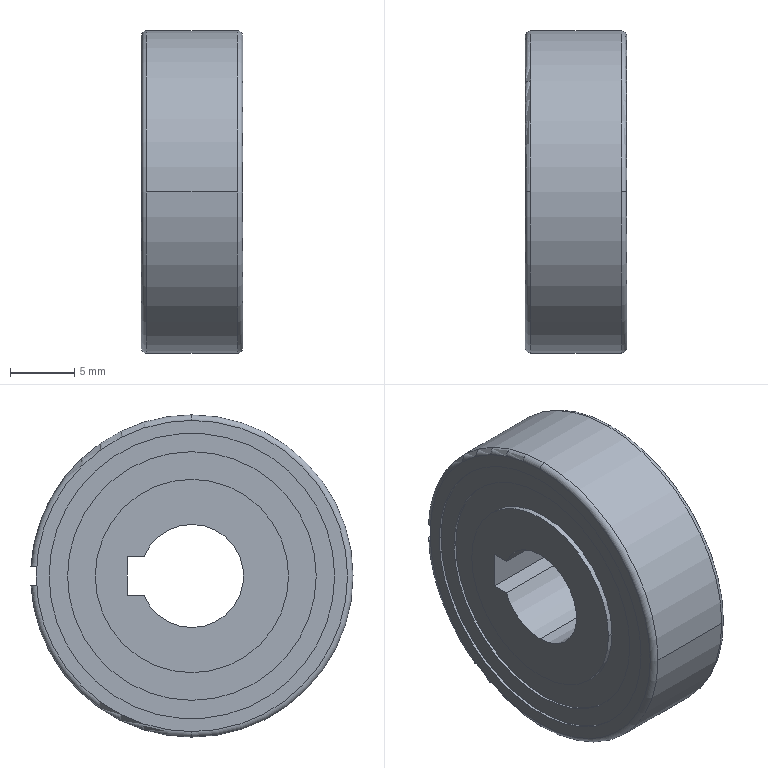Part | SolidWorks | features ICE 3, BaseBody 1, Scale 1 | 1 solid | 37 faces | box 7.854 x 24.97 x 24.99 mm | volume 3293 mm3 | cylinder 17 | plane 14 | torus 6 | commonest cylinder face diameters 14.994 x4 19.278 x4 22.134 x4 8 x3 24.99 x2
STEP:
#1=CARTESIAN_POINT('',(-3.927,-0.02811,4.));
#2=VERTEX_POINT('',#1);
#3=CARTESIAN_POINT('',(-3.927,-0.02811,-4.));
#4=VERTEX_POINT('',#3);
#5=CARTESIAN_POINT('',(-3.927,-0.02811,0.));
#6=DIRECTION('',(1.,0.,0.));
#7=DIRECTION('',(0.,0.,1.));
#8=AXIS2_PLACEMENT_3D('',#5,#6,#7);
#9=CIRCLE('',#8,4.);
#10=EDGE_CURVE('',#2,#4,#9,.T.);
#11=ORIENTED_EDGE('',*,*,#10,.F.);
#12=CARTESIAN_POINT('',(3.927,-0.02811,4.));
#13=VERTEX_POINT('',#12);
#14=CARTESIAN_POINT('',(-19.691,-0.02811,4.));
#15=DIRECTION('',(1.,0.,0.));
#16=VECTOR('',#15,1000.);
#17=LINE('',#14,#16);
#18=EDGE_CURVE('',#2,#13,#17,.T.);
#19=ORIENTED_EDGE('',*,*,#18,.T.);
#20=CARTESIAN_POINT('',(3.927,-0.02811,-4.));
#21=VERTEX_POINT('',#20);
#22=CARTESIAN_POINT('',(3.927,-0.02811,0.));
#23=DIRECTION('',(1.,0.,0.));
#24=DIRECTION('',(0.,0.,-1.));
#25=AXIS2_PLACEMENT_3D('',#22,#23,#24);
#26=CIRCLE('',#25,4.);
#27=EDGE_CURVE('',#13,#21,#26,.T.);
#28=ORIENTED_EDGE('',*,*,#27,.T.);
#29=CARTESIAN_POINT('',(-19.691,-0.02811,-4.));
#30=DIRECTION('',(1.,0.,0.));
#31=VECTOR('',#30,1000.);
#32=LINE('',#29,#31);
#33=EDGE_CURVE('',#4,#21,#32,.T.);
#34=ORIENTED_EDGE('',*,*,#33,.F.);
#35=EDGE_LOOP('',(#11,#19,#28,#34));
#36=FACE_OUTER_BOUND('',#35,.T.);
#37=CARTESIAN_POINT('',(-19.691,-0.02811,0.));
#38=DIRECTION('',(1.,0.,0.));
#39=DIRECTION('',(0.,0.,-1.));
#40=AXIS2_PLACEMENT_3D('',#37,#38,#39);
#41=CYLINDRICAL_SURFACE('',#40,4.);
#42=ADVANCED_FACE('',(#36),#41,.F.);
#43=CARTESIAN_POINT('',(-3.927,3.68,-1.5));
#44=VERTEX_POINT('',#43);
#45=CARTESIAN_POINT('',(-3.927,-0.02811,0.));
#46=DIRECTION('',(1.,0.,0.));
#47=DIRECTION('',(0.,0.,1.));
#48=AXIS2_PLACEMENT_3D('',#45,#46,#47);
#49=CIRCLE('',#48,4.);
#50=EDGE_CURVE('',#4,#44,#49,.T.);
#51=ORIENTED_EDGE('',*,*,#50,.F.);
#52=ORIENTED_EDGE('',*,*,#33,.T.);
#53=CARTESIAN_POINT('',(3.927,3.68,-1.5));
#54=VERTEX_POINT('',#53);
#55=CARTESIAN_POINT('',(3.927,-0.02811,0.));
#56=DIRECTION('',(1.,0.,0.));
#57=DIRECTION('',(0.,0.,-1.));
#58=AXIS2_PLACEMENT_3D('',#55,#56,#57);
#59=CIRCLE('',#58,4.);
#60=EDGE_CURVE('',#21,#54,#59,.T.);
#61=ORIENTED_EDGE('',*,*,#60,.T.);
#62=CARTESIAN_POINT('',(-19.691,3.68,-1.5));
#63=DIRECTION('',(-1.,0.,0.));
#64=VECTOR('',#63,1000.);
#65=LINE('',#62,#64);
#66=EDGE_CURVE('',#54,#44,#65,.T.);
#67=ORIENTED_EDGE('',*,*,#66,.T.);
#68=EDGE_LOOP('',(#51,#52,#61,#67));
#69=FACE_OUTER_BOUND('',#68,.T.);
#70=CARTESIAN_POINT('',(-19.691,-0.02811,0.));
#71=DIRECTION('',(1.,0.,0.));
#72=DIRECTION('',(0.,0.,-1.));
#73=AXIS2_PLACEMENT_3D('',#70,#71,#72);
#74=CYLINDRICAL_SURFACE('',#73,4.);
#75=ADVANCED_FACE('',(#69),#74,.F.);
#76=CARTESIAN_POINT('',(3.927,11.039,0.));
#77=VERTEX_POINT('',#76);
#78=CARTESIAN_POINT('',(3.927,-11.095,0.));
#79=VERTEX_POINT('',#78);
#80=CARTESIAN_POINT('',(3.927,-0.02811,0.));
#81=DIRECTION('',(-1.,0.,0.));
#82=DIRECTION('',(0.,1.,0.));
#83=AXIS2_PLACEMENT_3D('',#80,#81,#82);
#84=CIRCLE('',#83,11.067);
#85=EDGE_CURVE('',#77,#79,#84,.T.);
#86=ORIENTED_EDGE('',*,*,#85,.T.);
#87=CARTESIAN_POINT('',(3.927,-0.02811,0.));
#88=DIRECTION('',(-1.,0.,0.));
#89=DIRECTION('',(0.,1.,0.));
#90=AXIS2_PLACEMENT_3D('',#87,#88,#89);
#91=CIRCLE('',#90,11.067);
#92=EDGE_CURVE('',#79,#77,#91,.T.);
#93=ORIENTED_EDGE('',*,*,#92,.T.);
#94=EDGE_LOOP('',(#86,#93));
#95=FACE_BOUND('',#94,.T.);
#96=CARTESIAN_POINT('',(3.927,12.038,0.));
#97=VERTEX_POINT('',#96);
#98=CARTESIAN_POINT('',(3.927,-0.02811,-12.067));
#99=VERTEX_POINT('',#98);
#100=CARTESIAN_POINT('',(3.927,-0.02811,0.));
#101=DIRECTION('',(-1.,0.,0.));
#102=DIRECTION('',(0.,1.,0.));
#103=AXIS2_PLACEMENT_3D('',#100,#101,#102);
#104=CIRCLE('',#103,12.067);
#105=EDGE_CURVE('',#97,#99,#104,.T.);
#106=ORIENTED_EDGE('',*,*,#105,.F.);
#107=CARTESIAN_POINT('',(3.927,-0.02811,12.067));
#108=VERTEX_POINT('',#107);
#109=CARTESIAN_POINT('',(3.927,-0.02811,0.));
#110=DIRECTION('',(-1.,0.,0.));
#111=DIRECTION('',(0.,1.,0.));
#112=AXIS2_PLACEMENT_3D('',#109,#110,#111);
#113=CIRCLE('',#112,12.067);
#114=EDGE_CURVE('',#108,#97,#113,.T.);
#115=ORIENTED_EDGE('',*,*,#114,.F.);
#116=CARTESIAN_POINT('',(3.927,-0.02811,0.));
#117=DIRECTION('',(-1.,0.,0.));
#118=DIRECTION('',(0.,1.,0.));
#119=AXIS2_PLACEMENT_3D('',#116,#117,#118);
#120=CIRCLE('',#119,12.067);
#121=EDGE_CURVE('',#99,#108,#120,.T.);
#122=ORIENTED_EDGE('',*,*,#121,.F.);
#123=EDGE_LOOP('',(#106,#115,#122));
#124=FACE_OUTER_BOUND('',#123,.T.);
#125=CARTESIAN_POINT('',(3.927,11.539,0.));
#126=DIRECTION('',(1.,0.,0.));
#127=DIRECTION('',(0.,1.,0.));
#128=AXIS2_PLACEMENT_3D('',#125,#126,#127);
#129=PLANE('',#128);
#130=ADVANCED_FACE('',(#95,#124),#129,.T.);
#131=CARTESIAN_POINT('',(3.731,11.039,0.));
#132=VERTEX_POINT('',#131);
#133=CARTESIAN_POINT('',(3.829,11.039,0.));
#134=DIRECTION('',(-1.,0.,0.));
#135=VECTOR('',#134,1000.);
#136=LINE('',#133,#135);
#137=EDGE_CURVE('',#77,#132,#136,.T.);
#138=ORIENTED_EDGE('',*,*,#137,.T.);
#139=CARTESIAN_POINT('',(3.731,-11.095,0.));
#140=VERTEX_POINT('',#139);
#141=CARTESIAN_POINT('',(3.731,-0.02811,0.));
#142=DIRECTION('',(-1.,0.,0.));
#143=DIRECTION('',(0.,1.,0.));
#144=AXIS2_PLACEMENT_3D('',#141,#142,#143);
#145=CIRCLE('',#144,11.067);
#146=EDGE_CURVE('',#132,#140,#145,.T.);
#147=ORIENTED_EDGE('',*,*,#146,.T.);
#148=CARTESIAN_POINT('',(3.829,-11.095,0.));
#149=DIRECTION('',(1.,0.,0.));
#150=VECTOR('',#149,1000.);
#151=LINE('',#148,#150);
#152=EDGE_CURVE('',#140,#79,#151,.T.);
#153=ORIENTED_EDGE('',*,*,#152,.T.);
#154=ORIENTED_EDGE('',*,*,#85,.F.);
#155=EDGE_LOOP('',(#138,#147,#153,#154));
#156=FACE_OUTER_BOUND('',#155,.T.);
#157=CARTESIAN_POINT('',(3.829,-0.02811,0.));
#158=DIRECTION('',(-1.,0.,0.));
#159=DIRECTION('',(0.,1.,0.));
#160=AXIS2_PLACEMENT_3D('',#157,#158,#159);
#161=CYLINDRICAL_SURFACE('',#160,11.067);
#162=ADVANCED_FACE('',(#156),#161,.F.);
#163=CARTESIAN_POINT('',(3.731,9.611,0.));
#164=VERTEX_POINT('',#163);
#165=CARTESIAN_POINT('',(3.731,-9.667,0.));
#166=VERTEX_POINT('',#165);
#167=CARTESIAN_POINT('',(3.731,-0.02811,0.));
#168=DIRECTION('',(-1.,0.,0.));
#169=DIRECTION('',(0.,1.,0.));
#170=AXIS2_PLACEMENT_3D('',#167,#168,#169);
#171=CIRCLE('',#170,9.639);
#172=EDGE_CURVE('',#164,#166,#171,.T.);
#173=ORIENTED_EDGE('',*,*,#172,.T.);
#174=CARTESIAN_POINT('',(3.731,-0.02811,0.));
#175=DIRECTION('',(-1.,0.,0.));
#176=DIRECTION('',(0.,1.,0.));
#177=AXIS2_PLACEMENT_3D('',#174,#175,#176);
#178=CIRCLE('',#177,9.639);
#179=EDGE_CURVE('',#166,#164,#178,.T.);
#180=ORIENTED_EDGE('',*,*,#179,.T.);
#181=EDGE_LOOP('',(#173,#180));
#182=FACE_BOUND('',#181,.T.);
#183=ORIENTED_EDGE('',*,*,#146,.F.);
#184=CARTESIAN_POINT('',(3.731,-0.02811,0.));
#185=DIRECTION('',(-1.,0.,0.));
#186=DIRECTION('',(0.,1.,0.));
#187=AXIS2_PLACEMENT_3D('',#184,#185,#186);
#188=CIRCLE('',#187,11.067);
#189=EDGE_CURVE('',#140,#132,#188,.T.);
#190=ORIENTED_EDGE('',*,*,#189,.F.);
#191=EDGE_LOOP('',(#183,#190));
#192=FACE_OUTER_BOUND('',#191,.T.);
#193=CARTESIAN_POINT('',(3.731,10.325,0.));
#194=DIRECTION('',(1.,0.,0.));
#195=DIRECTION('',(0.,1.,0.));
#196=AXIS2_PLACEMENT_3D('',#193,#194,#195);
#197=PLANE('',#196);
#198=ADVANCED_FACE('',(#182,#192),#197,.T.);
#199=CARTESIAN_POINT('',(3.534,9.611,0.));
#200=VERTEX_POINT('',#199);
#201=CARTESIAN_POINT('',(3.632,9.611,0.));
#202=DIRECTION('',(-1.,0.,0.));
#203=VECTOR('',#202,1000.);
#204=LINE('',#201,#203);
#205=EDGE_CURVE('',#164,#200,#204,.T.);
#206=ORIENTED_EDGE('',*,*,#205,.T.);
#207=CARTESIAN_POINT('',(3.534,-9.667,0.));
#208=VERTEX_POINT('',#207);
#209=CARTESIAN_POINT('',(3.534,-0.02811,0.));
#210=DIRECTION('',(-1.,0.,0.));
#211=DIRECTION('',(0.,1.,0.));
#212=AXIS2_PLACEMENT_3D('',#209,#210,#211);
#213=CIRCLE('',#212,9.639);
#214=EDGE_CURVE('',#200,#208,#213,.T.);
#215=ORIENTED_EDGE('',*,*,#214,.T.);
#216=CARTESIAN_POINT('',(3.632,-9.667,0.));
#217=DIRECTION('',(1.,0.,0.));
#218=VECTOR('',#217,1000.);
#219=LINE('',#216,#218);
#220=EDGE_CURVE('',#208,#166,#219,.T.);
#221=ORIENTED_EDGE('',*,*,#220,.T.);
#222=ORIENTED_EDGE('',*,*,#172,.F.);
#223=EDGE_LOOP('',(#206,#215,#221,#222));
#224=FACE_OUTER_BOUND('',#223,.T.);
#225=CARTESIAN_POINT('',(3.632,-0.02811,0.));
#226=DIRECTION('',(-1.,0.,0.));
#227=DIRECTION('',(0.,1.,0.));
#228=AXIS2_PLACEMENT_3D('',#225,#226,#227);
#229=CYLINDRICAL_SURFACE('',#228,9.639);
#230=ADVANCED_FACE('',(#224),#229,.F.);
#231=CARTESIAN_POINT('',(3.534,7.469,0.));
#232=VERTEX_POINT('',#231);
#233=CARTESIAN_POINT('',(3.534,-7.525,0.));
#234=VERTEX_POINT('',#233);
#235=CARTESIAN_POINT('',(3.534,-0.02811,0.));
#236=DIRECTION('',(-1.,0.,0.));
#237=DIRECTION('',(0.,1.,0.));
#238=AXIS2_PLACEMENT_3D('',#235,#236,#237);
#239=CIRCLE('',#238,7.497);
#240=EDGE_CURVE('',#232,#234,#239,.T.);
#241=ORIENTED_EDGE('',*,*,#240,.T.);
#242=CARTESIAN_POINT('',(3.534,-0.02811,0.));
#243=DIRECTION('',(-1.,0.,0.));
#244=DIRECTION('',(0.,1.,0.));
#245=AXIS2_PLACEMENT_3D('',#242,#243,#244);
#246=CIRCLE('',#245,7.497);
#247=EDGE_CURVE('',#234,#232,#246,.T.);
#248=ORIENTED_EDGE('',*,*,#247,.T.);
#249=EDGE_LOOP('',(#241,#248));
#250=FACE_BOUND('',#249,.T.);
#251=ORIENTED_EDGE('',*,*,#214,.F.);
#252=CARTESIAN_POINT('',(3.534,-0.02811,0.));
#253=DIRECTION('',(-1.,0.,0.));
#254=DIRECTION('',(0.,1.,0.));
#255=AXIS2_PLACEMENT_3D('',#252,#253,#254);
#256=CIRCLE('',#255,9.639);
#257=EDGE_CURVE('',#208,#200,#256,.T.);
#258=ORIENTED_EDGE('',*,*,#257,.F.);
#259=EDGE_LOOP('',(#251,#258));
#260=FACE_OUTER_BOUND('',#259,.T.);
#261=CARTESIAN_POINT('',(3.534,8.54,0.));
#262=DIRECTION('',(1.,0.,0.));
#263=DIRECTION('',(0.,1.,0.));
#264=AXIS2_PLACEMENT_3D('',#261,#262,#263);
#265=PLANE('',#264);
#266=ADVANCED_FACE('',(#250,#260),#265,.T.);
#267=CARTESIAN_POINT('',(3.927,7.469,0.));
#268=VERTEX_POINT('',#267);
#269=CARTESIAN_POINT('',(3.731,7.469,0.));
#270=DIRECTION('',(-1.,0.,0.));
#271=VECTOR('',#270,1000.);
#272=LINE('',#269,#271);
#273=EDGE_CURVE('',#268,#232,#272,.T.);
#274=ORIENTED_EDGE('',*,*,#273,.T.);
#275=ORIENTED_EDGE('',*,*,#247,.F.);
#276=CARTESIAN_POINT('',(3.927,-7.525,0.));
#277=VERTEX_POINT('',#276);
#278=CARTESIAN_POINT('',(3.731,-7.525,0.));
#279=DIRECTION('',(1.,0.,0.));
#280=VECTOR('',#279,1000.);
#281=LINE('',#278,#280);
#282=EDGE_CURVE('',#234,#277,#281,.T.);
#283=ORIENTED_EDGE('',*,*,#282,.T.);
#284=CARTESIAN_POINT('',(3.927,-0.02811,0.));
#285=DIRECTION('',(-1.,0.,0.));
#286=DIRECTION('',(0.,1.,0.));
#287=AXIS2_PLACEMENT_3D('',#284,#285,#286);
#288=CIRCLE('',#287,7.497);
#289=EDGE_CURVE('',#277,#268,#288,.T.);
#290=ORIENTED_EDGE('',*,*,#289,.T.);
#291=EDGE_LOOP('',(#274,#275,#283,#290));
#292=FACE_OUTER_BOUND('',#291,.T.);
#293=CARTESIAN_POINT('',(3.731,-0.02811,0.));
#294=DIRECTION('',(-1.,0.,0.));
#295=DIRECTION('',(0.,1.,0.));
#296=AXIS2_PLACEMENT_3D('',#293,#294,#295);
#297=CYLINDRICAL_SURFACE('',#296,7.497);
#298=ADVANCED_FACE('',(#292),#297,.T.);
#299=CARTESIAN_POINT('',(3.927,5.,-1.5));
#300=VERTEX_POINT('',#299);
#301=CARTESIAN_POINT('',(3.927,5.,-1.5));
#302=DIRECTION('',(0.,1.,0.));
#303=VECTOR('',#302,1000.);
#304=LINE('',#301,#303);
#305=EDGE_CURVE('',#54,#300,#304,.T.);
#306=ORIENTED_EDGE('',*,*,#305,.F.);
#307=ORIENTED_EDGE('',*,*,#60,.F.);
#308=ORIENTED_EDGE('',*,*,#27,.F.);
#309=CARTESIAN_POINT('',(3.927,3.68,1.5));
#310=VERTEX_POINT('',#309);
#311=CARTESIAN_POINT('',(3.927,-0.02811,0.));
#312=DIRECTION('',(1.,0.,0.));
#313=DIRECTION('',(0.,0.,-1.));
#314=AXIS2_PLACEMENT_3D('',#311,#312,#313);
#315=CIRCLE('',#314,4.);
#316=EDGE_CURVE('',#310,#13,#315,.T.);
#317=ORIENTED_EDGE('',*,*,#316,.F.);
#318=CARTESIAN_POINT('',(3.927,5.,1.5));
#319=VERTEX_POINT('',#318);
#320=CARTESIAN_POINT('',(3.927,5.,1.5));
#321=DIRECTION('',(0.,-1.,0.));
#322=VECTOR('',#321,1000.);
#323=LINE('',#320,#322);
#324=EDGE_CURVE('',#319,#310,#323,.T.);
#325=ORIENTED_EDGE('',*,*,#324,.F.);
#326=CARTESIAN_POINT('',(3.927,5.,1.5));
#327=DIRECTION('',(0.,0.,1.));
#328=VECTOR('',#327,1000.);
#329=LINE('',#326,#328);
#330=EDGE_CURVE('',#300,#319,#329,.T.);
#331=ORIENTED_EDGE('',*,*,#330,.F.);
#332=EDGE_LOOP('',(#306,#307,#308,#317,#325,#331));
#333=FACE_BOUND('',#332,.T.);
#334=CARTESIAN_POINT('',(3.927,-0.02811,0.));
#335=DIRECTION('',(-1.,0.,0.));
#336=DIRECTION('',(0.,1.,0.));
#337=AXIS2_PLACEMENT_3D('',#334,#335,#336);
#338=CIRCLE('',#337,7.497);
#339=EDGE_CURVE('',#268,#277,#338,.T.);
#340=ORIENTED_EDGE('',*,*,#339,.F.);
#341=ORIENTED_EDGE('',*,*,#289,.F.);
#342=EDGE_LOOP('',(#340,#341));
#343=FACE_OUTER_BOUND('',#342,.T.);
#344=CARTESIAN_POINT('',(3.927,6.612,0.));
#345=DIRECTION('',(1.,0.,0.));
#346=DIRECTION('',(0.,1.,0.));
#347=AXIS2_PLACEMENT_3D('',#344,#345,#346);
#348=PLANE('',#347);
#349=ADVANCED_FACE('',(#333,#343),#348,.T.);
#350=CARTESIAN_POINT('',(-3.534,7.469,0.));
#351=VERTEX_POINT('',#350);
#352=CARTESIAN_POINT('',(-3.927,7.469,0.));
#353=VERTEX_POINT('',#352);
#354=CARTESIAN_POINT('',(-3.731,7.469,0.));
#355=DIRECTION('',(-1.,0.,0.));
#356=VECTOR('',#355,1000.);
#357=LINE('',#354,#356);
#358=EDGE_CURVE('',#351,#353,#357,.T.);
#359=ORIENTED_EDGE('',*,*,#358,.T.);
#360=CARTESIAN_POINT('',(-3.927,-7.525,0.));
#361=VERTEX_POINT('',#360);
#362=CARTESIAN_POINT('',(-3.927,-0.02811,0.));
#363=DIRECTION('',(-1.,0.,0.));
#364=DIRECTION('',(0.,1.,0.));
#365=AXIS2_PLACEMENT_3D('',#362,#363,#364);
#366=CIRCLE('',#365,7.497);
#367=EDGE_CURVE('',#361,#353,#366,.T.);
#368=ORIENTED_EDGE('',*,*,#367,.F.);
#369=CARTESIAN_POINT('',(-3.534,-7.525,0.));
#370=VERTEX_POINT('',#369);
#371=CARTESIAN_POINT('',(-3.731,-7.525,0.));
#372=DIRECTION('',(1.,0.,0.));
#373=VECTOR('',#372,1000.);
#374=LINE('',#371,#373);
#375=EDGE_CURVE('',#361,#370,#374,.T.);
#376=ORIENTED_EDGE('',*,*,#375,.T.);
#377=CARTESIAN_POINT('',(-3.534,-0.02811,0.));
#378=DIRECTION('',(-1.,0.,0.));
#379=DIRECTION('',(0.,1.,0.));
#380=AXIS2_PLACEMENT_3D('',#377,#378,#379);
#381=CIRCLE('',#380,7.497);
#382=EDGE_CURVE('',#370,#351,#381,.T.);
#383=ORIENTED_EDGE('',*,*,#382,.T.);
#384=EDGE_LOOP('',(#359,#368,#376,#383));
#385=FACE_OUTER_BOUND('',#384,.T.);
#386=CARTESIAN_POINT('',(-3.731,-0.02811,0.));
#387=DIRECTION('',(-1.,0.,0.));
#388=DIRECTION('',(0.,1.,0.));
#389=AXIS2_PLACEMENT_3D('',#386,#387,#388);
#390=CYLINDRICAL_SURFACE('',#389,7.497);
#391=ADVANCED_FACE('',(#385),#390,.T.);
#392=CARTESIAN_POINT('',(-3.534,-0.02811,0.));
#393=DIRECTION('',(-1.,0.,0.));
#394=DIRECTION('',(0.,1.,0.));
#395=AXIS2_PLACEMENT_3D('',#392,#393,#394);
#396=CIRCLE('',#395,7.497);
#397=EDGE_CURVE('',#351,#370,#396,.T.);
#398=ORIENTED_EDGE('',*,*,#397,.F.);
#399=ORIENTED_EDGE('',*,*,#382,.F.);
#400=EDGE_LOOP('',(#398,#399));
#401=FACE_BOUND('',#400,.T.);
#402=CARTESIAN_POINT('',(-3.534,9.611,0.));
#403=VERTEX_POINT('',#402);
#404=CARTESIAN_POINT('',(-3.534,-9.667,0.));
#405=VERTEX_POINT('',#404);
#406=CARTESIAN_POINT('',(-3.534,-0.02811,0.));
#407=DIRECTION('',(-1.,0.,0.));
#408=DIRECTION('',(0.,1.,0.));
#409=AXIS2_PLACEMENT_3D('',#406,#407,#408);
#410=CIRCLE('',#409,9.639);
#411=EDGE_CURVE('',#403,#405,#410,.T.);
#412=ORIENTED_EDGE('',*,*,#411,.T.);
#413=CARTESIAN_POINT('',(-3.534,-0.02811,0.));
#414=DIRECTION('',(-1.,0.,0.));
#415=DIRECTION('',(0.,1.,0.));
#416=AXIS2_PLACEMENT_3D('',#413,#414,#415);
#417=CIRCLE('',#416,9.639);
#418=EDGE_CURVE('',#405,#403,#417,.T.);
#419=ORIENTED_EDGE('',*,*,#418,.T.);
#420=EDGE_LOOP('',(#412,#419));
#421=FACE_OUTER_BOUND('',#420,.T.);
#422=CARTESIAN_POINT('',(-3.534,8.54,0.));
#423=DIRECTION('',(-1.,0.,0.));
#424=DIRECTION('',(0.,0.,1.));
#425=AXIS2_PLACEMENT_3D('',#422,#423,#424);
#426=PLANE('',#425);
#427=ADVANCED_FACE('',(#401,#421),#426,.T.);
#428=CARTESIAN_POINT('',(-3.731,9.611,0.));
#429=VERTEX_POINT('',#428);
#430=CARTESIAN_POINT('',(-3.632,9.611,0.));
#431=DIRECTION('',(-1.,0.,0.));
#432=VECTOR('',#431,1000.);
#433=LINE('',#430,#432);
#434=EDGE_CURVE('',#403,#429,#433,.T.);
#435=ORIENTED_EDGE('',*,*,#434,.T.);
#436=CARTESIAN_POINT('',(-3.731,-9.667,0.));
#437=VERTEX_POINT('',#436);
#438=CARTESIAN_POINT('',(-3.731,-0.02811,0.));
#439=DIRECTION('',(-1.,0.,0.));
#440=DIRECTION('',(0.,1.,0.));
#441=AXIS2_PLACEMENT_3D('',#438,#439,#440);
#442=CIRCLE('',#441,9.639);
#443=EDGE_CURVE('',#429,#437,#442,.T.);
#444=ORIENTED_EDGE('',*,*,#443,.T.);
#445=CARTESIAN_POINT('',(-3.632,-9.667,0.));
#446=DIRECTION('',(1.,0.,0.));
#447=VECTOR('',#446,1000.);
#448=LINE('',#445,#447);
#449=EDGE_CURVE('',#437,#405,#448,.T.);
#450=ORIENTED_EDGE('',*,*,#449,.T.);
#451=ORIENTED_EDGE('',*,*,#411,.F.);
#452=EDGE_LOOP('',(#435,#444,#450,#451));
#453=FACE_OUTER_BOUND('',#452,.T.);
#454=CARTESIAN_POINT('',(-3.632,-0.02811,0.));
#455=DIRECTION('',(-1.,0.,0.));
#456=DIRECTION('',(0.,1.,0.));
#457=AXIS2_PLACEMENT_3D('',#454,#455,#456);
#458=CYLINDRICAL_SURFACE('',#457,9.639);
#459=ADVANCED_FACE('',(#453),#458,.F.);
#460=ORIENTED_EDGE('',*,*,#443,.F.);
#461=CARTESIAN_POINT('',(-3.731,-0.02811,0.));
#462=DIRECTION('',(-1.,0.,0.));
#463=DIRECTION('',(0.,1.,0.));
#464=AXIS2_PLACEMENT_3D('',#461,#462,#463);
#465=CIRCLE('',#464,9.639);
#466=EDGE_CURVE('',#437,#429,#465,.T.);
#467=ORIENTED_EDGE('',*,*,#466,.F.);
#468=EDGE_LOOP('',(#460,#467));
#469=FACE_BOUND('',#468,.T.);
#470=CARTESIAN_POINT('',(-3.731,11.039,0.));
#471=VERTEX_POINT('',#470);
#472=CARTESIAN_POINT('',(-3.731,-11.095,0.));
#473=VERTEX_POINT('',#472);
#474=CARTESIAN_POINT('',(-3.731,-0.02811,0.));
#475=DIRECTION('',(-1.,0.,0.));
#476=DIRECTION('',(0.,1.,0.));
#477=AXIS2_PLACEMENT_3D('',#474,#475,#476);
#478=CIRCLE('',#477,11.067);
#479=EDGE_CURVE('',#471,#473,#478,.T.);
#480=ORIENTED_EDGE('',*,*,#479,.T.);
#481=CARTESIAN_POINT('',(-3.731,-0.02811,0.));
#482=DIRECTION('',(-1.,0.,0.));
#483=DIRECTION('',(0.,1.,0.));
#484=AXIS2_PLACEMENT_3D('',#481,#482,#483);
#485=CIRCLE('',#484,11.067);
#486=EDGE_CURVE('',#473,#471,#485,.T.);
#487=ORIENTED_EDGE('',*,*,#486,.T.);
#488=EDGE_LOOP('',(#480,#487));
#489=FACE_OUTER_BOUND('',#488,.T.);
#490=CARTESIAN_POINT('',(-3.731,10.325,0.));
#491=DIRECTION('',(-1.,0.,0.));
#492=DIRECTION('',(0.,0.,1.));
#493=AXIS2_PLACEMENT_3D('',#490,#491,#492);
#494=PLANE('',#493);
#495=ADVANCED_FACE('',(#469,#489),#494,.T.);
#496=CARTESIAN_POINT('',(-3.927,11.039,0.));
#497=VERTEX_POINT('',#496);
#498=CARTESIAN_POINT('',(-3.829,11.039,0.));
#499=DIRECTION('',(-1.,0.,0.));
#500=VECTOR('',#499,1000.);
#501=LINE('',#498,#500);
#502=EDGE_CURVE('',#471,#497,#501,.T.);
#503=ORIENTED_EDGE('',*,*,#502,.T.);
#504=CARTESIAN_POINT('',(-3.927,-11.095,0.));
#505=VERTEX_POINT('',#504);
#506=CARTESIAN_POINT('',(-3.927,-0.02811,0.));
#507=DIRECTION('',(-1.,0.,0.));
#508=DIRECTION('',(0.,1.,0.));
#509=AXIS2_PLACEMENT_3D('',#506,#507,#508);
#510=CIRCLE('',#509,11.067);
#511=EDGE_CURVE('',#497,#505,#510,.T.);
#512=ORIENTED_EDGE('',*,*,#511,.T.);
#513=CARTESIAN_POINT('',(-3.829,-11.095,0.));
#514=DIRECTION('',(1.,0.,0.));
#515=VECTOR('',#514,1000.);
#516=LINE('',#513,#515);
#517=EDGE_CURVE('',#505,#473,#516,.T.);
#518=ORIENTED_EDGE('',*,*,#517,.T.);
#519=ORIENTED_EDGE('',*,*,#479,.F.);
#520=EDGE_LOOP('',(#503,#512,#518,#519));
#521=FACE_OUTER_BOUND('',#520,.T.);
#522=CARTESIAN_POINT('',(-3.829,-0.02811,0.));
#523=DIRECTION('',(-1.,0.,0.));
#524=DIRECTION('',(0.,1.,0.));
#525=AXIS2_PLACEMENT_3D('',#522,#523,#524);
#526=CYLINDRICAL_SURFACE('',#525,11.067);
#527=ADVANCED_FACE('',(#521),#526,.F.);
#528=ORIENTED_EDGE('',*,*,#511,.F.);
#529=CARTESIAN_POINT('',(-3.927,-0.02811,0.));
#530=DIRECTION('',(-1.,0.,0.));
#531=DIRECTION('',(0.,1.,0.));
#532=AXIS2_PLACEMENT_3D('',#529,#530,#531);
#533=CIRCLE('',#532,11.067);
#534=EDGE_CURVE('',#505,#497,#533,.T.);
#535=ORIENTED_EDGE('',*,*,#534,.F.);
#536=EDGE_LOOP('',(#528,#535));
#537=FACE_BOUND('',#536,.T.);
#538=CARTESIAN_POINT('',(-3.927,12.038,0.));
#539=VERTEX_POINT('',#538);
#540=CARTESIAN_POINT('',(-3.927,-0.02811,-12.067));
#541=VERTEX_POINT('',#540);
#542=CARTESIAN_POINT('',(-3.927,-0.02811,0.));
#543=DIRECTION('',(-1.,0.,0.));
#544=DIRECTION('',(0.,1.,0.));
#545=AXIS2_PLACEMENT_3D('',#542,#543,#544);
#546=CIRCLE('',#545,12.067);
#547=EDGE_CURVE('',#539,#541,#546,.T.);
#548=ORIENTED_EDGE('',*,*,#547,.T.);
#549=CARTESIAN_POINT('',(-3.927,-0.02811,12.067));
#550=VERTEX_POINT('',#549);
#551=CARTESIAN_POINT('',(-3.927,-0.02811,0.));
#552=DIRECTION('',(-1.,0.,0.));
#553=DIRECTION('',(0.,1.,0.));
#554=AXIS2_PLACEMENT_3D('',#551,#552,#553);
#555=CIRCLE('',#554,12.067);
#556=EDGE_CURVE('',#541,#550,#555,.T.);
#557=ORIENTED_EDGE('',*,*,#556,.T.);
#558=CARTESIAN_POINT('',(-3.927,-0.02811,0.));
#559=DIRECTION('',(-1.,0.,0.));
#560=DIRECTION('',(0.,1.,0.));
#561=AXIS2_PLACEMENT_3D('',#558,#559,#560);
#562=CIRCLE('',#561,12.067);
#563=EDGE_CURVE('',#550,#539,#562,.T.);
#564=ORIENTED_EDGE('',*,*,#563,.T.);
#565=EDGE_LOOP('',(#548,#557,#564));
#566=FACE_OUTER_BOUND('',#565,.T.);
#567=CARTESIAN_POINT('',(-3.927,11.539,0.));
#568=DIRECTION('',(-1.,0.,0.));
#569=DIRECTION('',(0.,0.,1.));
#570=AXIS2_PLACEMENT_3D('',#567,#568,#569);
#571=PLANE('',#570);
#572=ADVANCED_FACE('',(#537,#566),#571,.T.);
#573=CARTESIAN_POINT('',(-3.499,-0.02811,12.495));
#574=VERTEX_POINT('',#573);
#575=CARTESIAN_POINT('',(-3.499,-0.02811,12.067));
#576=DIRECTION('',(0.,-1.,0.));
#577=DIRECTION('',(0.,0.,1.));
#578=AXIS2_PLACEMENT_3D('',#575,#576,#577);
#579=CIRCLE('',#578,0.4284);
#580=EDGE_CURVE('',#574,#550,#579,.T.);
#581=ORIENTED_EDGE('',*,*,#580,.T.);
#582=ORIENTED_EDGE('',*,*,#556,.F.);
#583=CARTESIAN_POINT('',(-3.499,-0.02811,-12.495));
#584=VERTEX_POINT('',#583);
#585=CARTESIAN_POINT('',(-3.499,-0.02811,-12.067));
#586=DIRECTION('',(0.,-1.,0.));
#587=DIRECTION('',(0.,0.,-1.));
#588=AXIS2_PLACEMENT_3D('',#585,#586,#587);
#589=CIRCLE('',#588,0.4284);
#590=EDGE_CURVE('',#541,#584,#589,.T.);
#591=ORIENTED_EDGE('',*,*,#590,.T.);
#592=CARTESIAN_POINT('',(-3.499,-12.523,0.));
#593=VERTEX_POINT('',#592);
#594=CARTESIAN_POINT('',(-3.499,-0.02811,0.));
#595=DIRECTION('',(-1.,0.,0.));
#596=DIRECTION('',(0.,1.,0.));
#597=AXIS2_PLACEMENT_3D('',#594,#595,#596);
#598=CIRCLE('',#597,12.495);
#599=EDGE_CURVE('',#584,#593,#598,.T.);
#600=ORIENTED_EDGE('',*,*,#599,.T.);
#601=CARTESIAN_POINT('',(-3.499,-0.02811,0.));
#602=DIRECTION('',(-1.,0.,0.));
#603=DIRECTION('',(0.,1.,0.));
#604=AXIS2_PLACEMENT_3D('',#601,#602,#603);
#605=CIRCLE('',#604,12.495);
#606=EDGE_CURVE('',#593,#574,#605,.T.);
#607=ORIENTED_EDGE('',*,*,#606,.T.);
#608=EDGE_LOOP('',(#581,#582,#591,#600,#607));
#609=FACE_OUTER_BOUND('',#608,.T.);
#610=CARTESIAN_POINT('',(-3.499,-0.02811,0.));
#611=DIRECTION('',(-1.,0.,0.));
#612=DIRECTION('',(0.,0.,1.));
#613=AXIS2_PLACEMENT_3D('',#610,#611,#612);
#614=TOROIDAL_SURFACE('',#613,12.067,0.4284);
#615=ADVANCED_FACE('',(#609),#614,.T.);
#616=CARTESIAN_POINT('',(3.499,-12.523,0.));
#617=VERTEX_POINT('',#616);
#618=CARTESIAN_POINT('',(0.,-12.523,0.));
#619=DIRECTION('',(1.,0.,0.));
#620=VECTOR('',#619,1000.);
#621=LINE('',#618,#620);
#622=EDGE_CURVE('',#593,#617,#621,.T.);
#623=ORIENTED_EDGE('',*,*,#622,.T.);
#624=CARTESIAN_POINT('',(3.499,-0.02811,12.495));
#625=VERTEX_POINT('',#624);
#626=CARTESIAN_POINT('',(3.499,-0.02811,0.));
#627=DIRECTION('',(-1.,0.,0.));
#628=DIRECTION('',(0.,1.,0.));
#629=AXIS2_PLACEMENT_3D('',#626,#627,#628);
#630=CIRCLE('',#629,12.495);
#631=EDGE_CURVE('',#617,#625,#630,.T.);
#632=ORIENTED_EDGE('',*,*,#631,.T.);
#633=CARTESIAN_POINT('',(3.499,12.446,0.714));
#634=VERTEX_POINT('',#633);
#635=CARTESIAN_POINT('',(3.499,-0.02811,0.));
#636=DIRECTION('',(-1.,0.,0.));
#637=DIRECTION('',(0.,1.,0.));
#638=AXIS2_PLACEMENT_3D('',#635,#636,#637);
#639=CIRCLE('',#638,12.495);
#640=EDGE_CURVE('',#625,#634,#639,.T.);
#641=ORIENTED_EDGE('',*,*,#640,.T.);
#642=CARTESIAN_POINT('',(-3.499,12.446,0.714));
#643=VERTEX_POINT('',#642);
#644=CARTESIAN_POINT('',(0.,12.446,0.714));
#645=DIRECTION('',(-1.,0.,0.));
#646=VECTOR('',#645,1000.);
#647=LINE('',#644,#646);
#648=EDGE_CURVE('',#634,#643,#647,.T.);
#649=ORIENTED_EDGE('',*,*,#648,.T.);
#650=CARTESIAN_POINT('',(-3.499,-0.02811,0.));
#651=DIRECTION('',(-1.,0.,0.));
#652=DIRECTION('',(0.,1.,0.));
#653=AXIS2_PLACEMENT_3D('',#650,#651,#652);
#654=CIRCLE('',#653,12.495);
#655=EDGE_CURVE('',#574,#643,#654,.T.);
#656=ORIENTED_EDGE('',*,*,#655,.F.);
#657=ORIENTED_EDGE('',*,*,#606,.F.);
#658=EDGE_LOOP('',(#623,#632,#641,#649,#656,#657));
#659=FACE_OUTER_BOUND('',#658,.T.);
#660=CARTESIAN_POINT('',(0.,-0.02811,0.));
#661=DIRECTION('',(-1.,0.,0.));
#662=DIRECTION('',(0.,1.,0.));
#663=AXIS2_PLACEMENT_3D('',#660,#661,#662);
#664=CYLINDRICAL_SURFACE('',#663,12.495);
#665=ADVANCED_FACE('',(#659),#664,.T.);
#666=CARTESIAN_POINT('',(3.499,-0.02811,12.067));
#667=DIRECTION('',(0.,-1.,0.));
#668=DIRECTION('',(0.,0.,1.));
#669=AXIS2_PLACEMENT_3D('',#666,#667,#668);
#670=CIRCLE('',#669,0.4284);
#671=EDGE_CURVE('',#108,#625,#670,.T.);
#672=ORIENTED_EDGE('',*,*,#671,.T.);
#673=ORIENTED_EDGE('',*,*,#631,.F.);
#674=CARTESIAN_POINT('',(3.499,-0.02811,-12.495));
#675=VERTEX_POINT('',#674);
#676=CARTESIAN_POINT('',(3.499,-0.02811,0.));
#677=DIRECTION('',(-1.,0.,0.));
#678=DIRECTION('',(0.,1.,0.));
#679=AXIS2_PLACEMENT_3D('',#676,#677,#678);
#680=CIRCLE('',#679,12.495);
#681=EDGE_CURVE('',#675,#617,#680,.T.);
#682=ORIENTED_EDGE('',*,*,#681,.F.);
#683=CARTESIAN_POINT('',(3.499,-0.02811,-12.067));
#684=DIRECTION('',(0.,-1.,0.));
#685=DIRECTION('',(0.,0.,-1.));
#686=AXIS2_PLACEMENT_3D('',#683,#684,#685);
#687=CIRCLE('',#686,0.4284);
#688=EDGE_CURVE('',#675,#99,#687,.T.);
#689=ORIENTED_EDGE('',*,*,#688,.T.);
#690=ORIENTED_EDGE('',*,*,#121,.T.);
#691=EDGE_LOOP('',(#672,#673,#682,#689,#690));
#692=FACE_OUTER_BOUND('',#691,.T.);
#693=CARTESIAN_POINT('',(3.499,-0.02811,0.));
#694=DIRECTION('',(-1.,0.,0.));
#695=DIRECTION('',(0.,0.,1.));
#696=AXIS2_PLACEMENT_3D('',#693,#694,#695);
#697=TOROIDAL_SURFACE('',#696,12.067,0.4284);
#698=ADVANCED_FACE('',(#692),#697,.T.);
#699=CARTESIAN_POINT('',(3.499,12.446,-0.714));
#700=VERTEX_POINT('',#699);
#701=CARTESIAN_POINT('',(3.926,12.038,-0.714));
#702=VERTEX_POINT('',#701);
#703=CARTESIAN_POINT('',(3.499,12.446,-0.714));
#704=CARTESIAN_POINT('',(3.584,12.446,-0.714));
#705=CARTESIAN_POINT('',(3.684,12.419,-0.7145));
#706=CARTESIAN_POINT('',(3.853,12.282,-0.7146));
#707=CARTESIAN_POINT('',(3.92,12.17,-0.714));
#708=CARTESIAN_POINT('',(3.926,12.038,-0.714));
#709=B_SPLINE_CURVE_WITH_KNOTS('',3,(#703,#704,#705,#706,#707,#708),.UNSPECIFIED.,.F.,.F.,(4,2,4),(0.,0.5,1.),.UNSPECIFIED.);
#710=EDGE_CURVE('',#700,#702,#709,.T.);
#711=ORIENTED_EDGE('',*,*,#710,.F.);
#712=CARTESIAN_POINT('',(-3.499,12.446,-0.714));
#713=VERTEX_POINT('',#712);
#714=CARTESIAN_POINT('',(0.,12.446,-0.714));
#715=DIRECTION('',(1.,0.,0.));
#716=VECTOR('',#715,1000.);
#717=LINE('',#714,#716);
#718=EDGE_CURVE('',#713,#700,#717,.T.);
#719=ORIENTED_EDGE('',*,*,#718,.F.);
#720=CARTESIAN_POINT('',(-3.926,12.038,-0.714));
#721=VERTEX_POINT('',#720);
#722=CARTESIAN_POINT('',(-3.926,12.038,-0.714));
#723=CARTESIAN_POINT('',(-3.92,12.17,-0.714));
#724=CARTESIAN_POINT('',(-3.853,12.282,-0.7146));
#725=CARTESIAN_POINT('',(-3.684,12.419,-0.7145));
#726=CARTESIAN_POINT('',(-3.584,12.446,-0.714));
#727=CARTESIAN_POINT('',(-3.499,12.446,-0.714));
#728=B_SPLINE_CURVE_WITH_KNOTS('',3,(#722,#723,#724,#725,#726,#727),.UNSPECIFIED.,.F.,.F.,(4,2,4),(0.,0.5,1.),.UNSPECIFIED.);
#729=EDGE_CURVE('',#721,#713,#728,.T.);
#730=ORIENTED_EDGE('',*,*,#729,.F.);
#731=CARTESIAN_POINT('',(-3.927,12.038,-0.714));
#732=DIRECTION('',(1.,0.,0.));
#733=VECTOR('',#732,1000.);
#734=LINE('',#731,#733);
#735=EDGE_CURVE('',#721,#702,#734,.T.);
#736=ORIENTED_EDGE('',*,*,#735,.T.);
#737=EDGE_LOOP('',(#711,#719,#730,#736));
#738=FACE_OUTER_BOUND('',#737,.T.);
#739=CARTESIAN_POINT('',(-3.927,12.242,-0.714));
#740=DIRECTION('',(0.,0.,-1.));
#741=DIRECTION('',(0.,-1.,0.));
#742=AXIS2_PLACEMENT_3D('',#739,#740,#741);
#743=PLANE('',#742);
#744=ADVANCED_FACE('',(#738),#743,.F.);
#745=CARTESIAN_POINT('',(3.926,12.038,-0.714));
#746=CARTESIAN_POINT('',(3.927,12.038,-0.4764));
#747=CARTESIAN_POINT('',(3.927,12.038,-0.2387));
#748=CARTESIAN_POINT('',(3.927,12.038,0.));
#749=B_SPLINE_CURVE_WITH_KNOTS('',3,(#745,#746,#747,#748),.UNSPECIFIED.,.F.,.F.,(4,4),(0.,1.),.UNSPECIFIED.);
#750=EDGE_CURVE('',#702,#97,#749,.T.);
#751=ORIENTED_EDGE('',*,*,#750,.F.);
#752=ORIENTED_EDGE('',*,*,#735,.F.);
#753=CARTESIAN_POINT('',(-3.927,12.038,0.));
#754=CARTESIAN_POINT('',(-3.927,12.038,-0.2387));
#755=CARTESIAN_POINT('',(-3.927,12.038,-0.4764));
#756=CARTESIAN_POINT('',(-3.926,12.038,-0.714));
#757=B_SPLINE_CURVE_WITH_KNOTS('',3,(#753,#754,#755,#756),.UNSPECIFIED.,.F.,.F.,(4,4),(0.,1.),.UNSPECIFIED.);
#758=EDGE_CURVE('',#539,#721,#757,.T.);
#759=ORIENTED_EDGE('',*,*,#758,.F.);
#760=CARTESIAN_POINT('',(-3.926,12.038,0.714));
#761=VERTEX_POINT('',#760);
#762=CARTESIAN_POINT('',(-3.926,12.038,0.714));
#763=CARTESIAN_POINT('',(-3.927,12.038,0.4764));
#764=CARTESIAN_POINT('',(-3.927,12.038,0.2387));
#765=CARTESIAN_POINT('',(-3.927,12.038,0.));
#766=B_SPLINE_CURVE_WITH_KNOTS('',3,(#762,#763,#764,#765),.UNSPECIFIED.,.F.,.F.,(4,4),(0.,1.),.UNSPECIFIED.);
#767=EDGE_CURVE('',#761,#539,#766,.T.);
#768=ORIENTED_EDGE('',*,*,#767,.F.);
#769=CARTESIAN_POINT('',(3.926,12.038,0.714));
#770=VERTEX_POINT('',#769);
#771=CARTESIAN_POINT('',(-3.927,12.038,0.714));
#772=DIRECTION('',(1.,0.,0.));
#773=VECTOR('',#772,1000.);
#774=LINE('',#771,#773);
#775=EDGE_CURVE('',#761,#770,#774,.T.);
#776=ORIENTED_EDGE('',*,*,#775,.T.);
#777=CARTESIAN_POINT('',(3.927,12.038,0.));
#778=CARTESIAN_POINT('',(3.927,12.038,0.2387));
#779=CARTESIAN_POINT('',(3.927,12.038,0.4764));
#780=CARTESIAN_POINT('',(3.926,12.038,0.714));
#781=B_SPLINE_CURVE_WITH_KNOTS('',3,(#777,#778,#779,#780),.UNSPECIFIED.,.F.,.F.,(4,4),(0.,1.),.UNSPECIFIED.);
#782=EDGE_CURVE('',#97,#770,#781,.T.);
#783=ORIENTED_EDGE('',*,*,#782,.F.);
#784=EDGE_LOOP('',(#751,#752,#759,#768,#776,#783));
#785=FACE_OUTER_BOUND('',#784,.T.);
#786=CARTESIAN_POINT('',(-3.927,12.038,0.));
#787=DIRECTION('',(0.,-1.,0.));
#788=DIRECTION('',(0.,0.,-1.));
#789=AXIS2_PLACEMENT_3D('',#786,#787,#788);
#790=PLANE('',#789);
#791=ADVANCED_FACE('',(#785),#790,.F.);
#792=CARTESIAN_POINT('',(3.926,12.038,0.714));
#793=CARTESIAN_POINT('',(3.92,12.17,0.714));
#794=CARTESIAN_POINT('',(3.853,12.282,0.7146));
#795=CARTESIAN_POINT('',(3.684,12.419,0.7145));
#796=CARTESIAN_POINT('',(3.584,12.446,0.714));
#797=CARTESIAN_POINT('',(3.499,12.446,0.714));
#798=B_SPLINE_CURVE_WITH_KNOTS('',3,(#792,#793,#794,#795,#796,#797),.UNSPECIFIED.,.F.,.F.,(4,2,4),(0.,0.5,1.),.UNSPECIFIED.);
#799=EDGE_CURVE('',#770,#634,#798,.T.);
#800=ORIENTED_EDGE('',*,*,#799,.F.);
#801=ORIENTED_EDGE('',*,*,#775,.F.);
#802=CARTESIAN_POINT('',(-3.499,12.446,0.714));
#803=CARTESIAN_POINT('',(-3.584,12.446,0.714));
#804=CARTESIAN_POINT('',(-3.684,12.419,0.7145));
#805=CARTESIAN_POINT('',(-3.853,12.282,0.7146));
#806=CARTESIAN_POINT('',(-3.92,12.17,0.714));
#807=CARTESIAN_POINT('',(-3.926,12.038,0.714));
#808=B_SPLINE_CURVE_WITH_KNOTS('',3,(#802,#803,#804,#805,#806,#807),.UNSPECIFIED.,.F.,.F.,(4,2,4),(0.,0.5,1.),.UNSPECIFIED.);
#809=EDGE_CURVE('',#643,#761,#808,.T.);
#810=ORIENTED_EDGE('',*,*,#809,.F.);
#811=ORIENTED_EDGE('',*,*,#648,.F.);
#812=EDGE_LOOP('',(#800,#801,#810,#811));
#813=FACE_OUTER_BOUND('',#812,.T.);
#814=CARTESIAN_POINT('',(-3.927,12.242,0.714));
#815=DIRECTION('',(0.,0.,1.));
#816=DIRECTION('',(1.,0.,0.));
#817=AXIS2_PLACEMENT_3D('',#814,#815,#816);
#818=PLANE('',#817);
#819=ADVANCED_FACE('',(#813),#818,.F.);
#820=CARTESIAN_POINT('',(-3.927,5.,-1.5));
#821=VERTEX_POINT('',#820);
#822=CARTESIAN_POINT('',(-3.927,5.,-1.5));
#823=DIRECTION('',(0.,1.,0.));
#824=VECTOR('',#823,1000.);
#825=LINE('',#822,#824);
#826=EDGE_CURVE('',#44,#821,#825,.T.);
#827=ORIENTED_EDGE('',*,*,#826,.T.);
#828=CARTESIAN_POINT('',(-3.927,5.,1.5));
#829=VERTEX_POINT('',#828);
#830=CARTESIAN_POINT('',(-3.927,5.,1.5));
#831=DIRECTION('',(0.,0.,1.));
#832=VECTOR('',#831,1000.);
#833=LINE('',#830,#832);
#834=EDGE_CURVE('',#821,#829,#833,.T.);
#835=ORIENTED_EDGE('',*,*,#834,.T.);
#836=CARTESIAN_POINT('',(-3.927,3.68,1.5));
#837=VERTEX_POINT('',#836);
#838=CARTESIAN_POINT('',(-3.927,5.,1.5));
#839=DIRECTION('',(0.,-1.,0.));
#840=VECTOR('',#839,1000.);
#841=LINE('',#838,#840);
#842=EDGE_CURVE('',#829,#837,#841,.T.);
#843=ORIENTED_EDGE('',*,*,#842,.T.);
#844=CARTESIAN_POINT('',(-3.927,-0.02811,0.));
#845=DIRECTION('',(1.,0.,0.));
#846=DIRECTION('',(0.,0.,1.));
#847=AXIS2_PLACEMENT_3D('',#844,#845,#846);
#848=CIRCLE('',#847,4.);
#849=EDGE_CURVE('',#837,#2,#848,.T.);
#850=ORIENTED_EDGE('',*,*,#849,.T.);
#851=ORIENTED_EDGE('',*,*,#10,.T.);
#852=ORIENTED_EDGE('',*,*,#50,.T.);
#853=EDGE_LOOP('',(#827,#835,#843,#850,#851,#852));
#854=FACE_BOUND('',#853,.T.);
#855=CARTESIAN_POINT('',(-3.927,-0.02811,0.));
#856=DIRECTION('',(-1.,0.,0.));
#857=DIRECTION('',(0.,1.,0.));
#858=AXIS2_PLACEMENT_3D('',#855,#856,#857);
#859=CIRCLE('',#858,7.497);
#860=EDGE_CURVE('',#353,#361,#859,.T.);
#861=ORIENTED_EDGE('',*,*,#860,.T.);
#862=ORIENTED_EDGE('',*,*,#367,.T.);
#863=EDGE_LOOP('',(#861,#862));
#864=FACE_OUTER_BOUND('',#863,.T.);
#865=CARTESIAN_POINT('',(-3.927,6.612,0.));
#866=DIRECTION('',(-1.,0.,0.));
#867=DIRECTION('',(0.,0.,1.));
#868=AXIS2_PLACEMENT_3D('',#865,#866,#867);
#869=PLANE('',#868);
#870=ADVANCED_FACE('',(#854,#864),#869,.T.);
#871=ORIENTED_EDGE('',*,*,#671,.F.);
#872=ORIENTED_EDGE('',*,*,#114,.T.);
#873=ORIENTED_EDGE('',*,*,#782,.T.);
#874=ORIENTED_EDGE('',*,*,#799,.T.);
#875=ORIENTED_EDGE('',*,*,#640,.F.);
#876=EDGE_LOOP('',(#871,#872,#873,#874,#875));
#877=FACE_OUTER_BOUND('',#876,.T.);
#878=CARTESIAN_POINT('',(3.499,-0.02811,0.));
#879=DIRECTION('',(-1.,0.,0.));
#880=DIRECTION('',(0.,0.,1.));
#881=AXIS2_PLACEMENT_3D('',#878,#879,#880);
#882=TOROIDAL_SURFACE('',#881,12.067,0.4284);
#883=ADVANCED_FACE('',(#877),#882,.T.);
#884=ORIENTED_EDGE('',*,*,#688,.F.);
#885=CARTESIAN_POINT('',(3.499,-0.02811,0.));
#886=DIRECTION('',(-1.,0.,0.));
#887=DIRECTION('',(0.,1.,0.));
#888=AXIS2_PLACEMENT_3D('',#885,#886,#887);
#889=CIRCLE('',#888,12.495);
#890=EDGE_CURVE('',#700,#675,#889,.T.);
#891=ORIENTED_EDGE('',*,*,#890,.F.);
#892=ORIENTED_EDGE('',*,*,#710,.T.);
#893=ORIENTED_EDGE('',*,*,#750,.T.);
#894=ORIENTED_EDGE('',*,*,#105,.T.);
#895=EDGE_LOOP('',(#884,#891,#892,#893,#894));
#896=FACE_OUTER_BOUND('',#895,.T.);
#897=CARTESIAN_POINT('',(3.499,-0.02811,0.));
#898=DIRECTION('',(-1.,0.,0.));
#899=DIRECTION('',(0.,0.,1.));
#900=AXIS2_PLACEMENT_3D('',#897,#898,#899);
#901=TOROIDAL_SURFACE('',#900,12.067,0.4284);
#902=ADVANCED_FACE('',(#896),#901,.T.);
#903=ORIENTED_EDGE('',*,*,#622,.F.);
#904=ORIENTED_EDGE('',*,*,#599,.F.);
#905=CARTESIAN_POINT('',(-3.499,-0.02811,0.));
#906=DIRECTION('',(-1.,0.,0.));
#907=DIRECTION('',(0.,1.,0.));
#908=AXIS2_PLACEMENT_3D('',#905,#906,#907);
#909=CIRCLE('',#908,12.495);
#910=EDGE_CURVE('',#713,#584,#909,.T.);
#911=ORIENTED_EDGE('',*,*,#910,.F.);
#912=ORIENTED_EDGE('',*,*,#718,.T.);
#913=ORIENTED_EDGE('',*,*,#890,.T.);
#914=ORIENTED_EDGE('',*,*,#681,.T.);
#915=EDGE_LOOP('',(#903,#904,#911,#912,#913,#914));
#916=FACE_OUTER_BOUND('',#915,.T.);
#917=CARTESIAN_POINT('',(0.,-0.02811,0.));
#918=DIRECTION('',(-1.,0.,0.));
#919=DIRECTION('',(0.,1.,0.));
#920=AXIS2_PLACEMENT_3D('',#917,#918,#919);
#921=CYLINDRICAL_SURFACE('',#920,12.495);
#922=ADVANCED_FACE('',(#916),#921,.T.);
#923=ORIENTED_EDGE('',*,*,#580,.F.);
#924=ORIENTED_EDGE('',*,*,#655,.T.);
#925=ORIENTED_EDGE('',*,*,#809,.T.);
#926=ORIENTED_EDGE('',*,*,#767,.T.);
#927=ORIENTED_EDGE('',*,*,#563,.F.);
#928=EDGE_LOOP('',(#923,#924,#925,#926,#927));
#929=FACE_OUTER_BOUND('',#928,.T.);
#930=CARTESIAN_POINT('',(-3.499,-0.02811,0.));
#931=DIRECTION('',(-1.,0.,0.));
#932=DIRECTION('',(0.,0.,1.));
#933=AXIS2_PLACEMENT_3D('',#930,#931,#932);
#934=TOROIDAL_SURFACE('',#933,12.067,0.4284);
#935=ADVANCED_FACE('',(#929),#934,.T.);
#936=ORIENTED_EDGE('',*,*,#590,.F.);
#937=ORIENTED_EDGE('',*,*,#547,.F.);
#938=ORIENTED_EDGE('',*,*,#758,.T.);
#939=ORIENTED_EDGE('',*,*,#729,.T.);
#940=ORIENTED_EDGE('',*,*,#910,.T.);
#941=EDGE_LOOP('',(#936,#937,#938,#939,#940));
#942=FACE_OUTER_BOUND('',#941,.T.);
#943=CARTESIAN_POINT('',(-3.499,-0.02811,0.));
#944=DIRECTION('',(-1.,0.,0.));
#945=DIRECTION('',(0.,0.,1.));
#946=AXIS2_PLACEMENT_3D('',#943,#944,#945);
#947=TOROIDAL_SURFACE('',#946,12.067,0.4284);
#948=ADVANCED_FACE('',(#942),#947,.T.);
#949=ORIENTED_EDGE('',*,*,#502,.F.);
#950=ORIENTED_EDGE('',*,*,#486,.F.);
#951=ORIENTED_EDGE('',*,*,#517,.F.);
#952=ORIENTED_EDGE('',*,*,#534,.T.);
#953=EDGE_LOOP('',(#949,#950,#951,#952));
#954=FACE_OUTER_BOUND('',#953,.T.);
#955=CARTESIAN_POINT('',(-3.829,-0.02811,0.));
#956=DIRECTION('',(-1.,0.,0.));
#957=DIRECTION('',(0.,1.,0.));
#958=AXIS2_PLACEMENT_3D('',#955,#956,#957);
#959=CYLINDRICAL_SURFACE('',#958,11.067);
#960=ADVANCED_FACE('',(#954),#959,.F.);
#961=ORIENTED_EDGE('',*,*,#434,.F.);
#962=ORIENTED_EDGE('',*,*,#418,.F.);
#963=ORIENTED_EDGE('',*,*,#449,.F.);
#964=ORIENTED_EDGE('',*,*,#466,.T.);
#965=EDGE_LOOP('',(#961,#962,#963,#964));
#966=FACE_OUTER_BOUND('',#965,.T.);
#967=CARTESIAN_POINT('',(-3.632,-0.02811,0.));
#968=DIRECTION('',(-1.,0.,0.));
#969=DIRECTION('',(0.,1.,0.));
#970=AXIS2_PLACEMENT_3D('',#967,#968,#969);
#971=CYLINDRICAL_SURFACE('',#970,9.639);
#972=ADVANCED_FACE('',(#966),#971,.F.);
#973=ORIENTED_EDGE('',*,*,#358,.F.);
#974=ORIENTED_EDGE('',*,*,#397,.T.);
#975=ORIENTED_EDGE('',*,*,#375,.F.);
#976=ORIENTED_EDGE('',*,*,#860,.F.);
#977=EDGE_LOOP('',(#973,#974,#975,#976));
#978=FACE_OUTER_BOUND('',#977,.T.);
#979=CARTESIAN_POINT('',(-3.731,-0.02811,0.));
#980=DIRECTION('',(-1.,0.,0.));
#981=DIRECTION('',(0.,1.,0.));
#982=AXIS2_PLACEMENT_3D('',#979,#980,#981);
#983=CYLINDRICAL_SURFACE('',#982,7.497);
#984=ADVANCED_FACE('',(#978),#983,.T.);
#985=ORIENTED_EDGE('',*,*,#273,.F.);
#986=ORIENTED_EDGE('',*,*,#339,.T.);
#987=ORIENTED_EDGE('',*,*,#282,.F.);
#988=ORIENTED_EDGE('',*,*,#240,.F.);
#989=EDGE_LOOP('',(#985,#986,#987,#988));
#990=FACE_OUTER_BOUND('',#989,.T.);
#991=CARTESIAN_POINT('',(3.731,-0.02811,0.));
#992=DIRECTION('',(-1.,0.,0.));
#993=DIRECTION('',(0.,1.,0.));
#994=AXIS2_PLACEMENT_3D('',#991,#992,#993);
#995=CYLINDRICAL_SURFACE('',#994,7.497);
#996=ADVANCED_FACE('',(#990),#995,.T.);
#997=ORIENTED_EDGE('',*,*,#205,.F.);
#998=ORIENTED_EDGE('',*,*,#179,.F.);
#999=ORIENTED_EDGE('',*,*,#220,.F.);
#1000=ORIENTED_EDGE('',*,*,#257,.T.);
#1001=EDGE_LOOP('',(#997,#998,#999,#1000));
#1002=FACE_OUTER_BOUND('',#1001,.T.);
#1003=CARTESIAN_POINT('',(3.632,-0.02811,0.));
#1004=DIRECTION('',(-1.,0.,0.));
#1005=DIRECTION('',(0.,1.,0.));
#1006=AXIS2_PLACEMENT_3D('',#1003,#1004,#1005);
#1007=CYLINDRICAL_SURFACE('',#1006,9.639);
#1008=ADVANCED_FACE('',(#1002),#1007,.F.);
#1009=ORIENTED_EDGE('',*,*,#137,.F.);
#1010=ORIENTED_EDGE('',*,*,#92,.F.);
#1011=ORIENTED_EDGE('',*,*,#152,.F.);
#1012=ORIENTED_EDGE('',*,*,#189,.T.);
#1013=EDGE_LOOP('',(#1009,#1010,#1011,#1012));
#1014=FACE_OUTER_BOUND('',#1013,.T.);
#1015=CARTESIAN_POINT('',(3.829,-0.02811,0.));
#1016=DIRECTION('',(-1.,0.,0.));
#1017=DIRECTION('',(0.,1.,0.));
#1018=AXIS2_PLACEMENT_3D('',#1015,#1016,#1017);
#1019=CYLINDRICAL_SURFACE('',#1018,11.067);
#1020=ADVANCED_FACE('',(#1014),#1019,.F.);
#1021=ORIENTED_EDGE('',*,*,#18,.F.);
#1022=ORIENTED_EDGE('',*,*,#849,.F.);
#1023=CARTESIAN_POINT('',(-19.691,3.68,1.5));
#1024=DIRECTION('',(1.,0.,0.));
#1025=VECTOR('',#1024,1000.);
#1026=LINE('',#1023,#1025);
#1027=EDGE_CURVE('',#837,#310,#1026,.T.);
#1028=ORIENTED_EDGE('',*,*,#1027,.T.);
#1029=ORIENTED_EDGE('',*,*,#316,.T.);
#1030=EDGE_LOOP('',(#1021,#1022,#1028,#1029));
#1031=FACE_OUTER_BOUND('',#1030,.T.);
#1032=CARTESIAN_POINT('',(-19.691,-0.02811,0.));
#1033=DIRECTION('',(1.,0.,0.));
#1034=DIRECTION('',(0.,0.,-1.));
#1035=AXIS2_PLACEMENT_3D('',#1032,#1033,#1034);
#1036=CYLINDRICAL_SURFACE('',#1035,4.);
#1037=ADVANCED_FACE('',(#1031),#1036,.F.);
#1038=ORIENTED_EDGE('',*,*,#305,.T.);
#1039=CARTESIAN_POINT('',(-8.17,5.,-1.5));
#1040=DIRECTION('',(1.,0.,0.));
#1041=VECTOR('',#1040,1000.);
#1042=LINE('',#1039,#1041);
#1043=EDGE_CURVE('',#821,#300,#1042,.T.);
#1044=ORIENTED_EDGE('',*,*,#1043,.F.);
#1045=ORIENTED_EDGE('',*,*,#826,.F.);
#1046=ORIENTED_EDGE('',*,*,#66,.F.);
#1047=EDGE_LOOP('',(#1038,#1044,#1045,#1046));
#1048=FACE_OUTER_BOUND('',#1047,.T.);
#1049=CARTESIAN_POINT('',(-8.17,5.,-1.5));
#1050=DIRECTION('',(0.,0.,-1.));
#1051=DIRECTION('',(0.,1.,0.));
#1052=AXIS2_PLACEMENT_3D('',#1049,#1050,#1051);
#1053=PLANE('',#1052);
#1054=ADVANCED_FACE('',(#1048),#1053,.F.);
#1055=ORIENTED_EDGE('',*,*,#842,.F.);
#1056=CARTESIAN_POINT('',(-8.17,5.,1.5));
#1057=DIRECTION('',(1.,0.,0.));
#1058=VECTOR('',#1057,1000.);
#1059=LINE('',#1056,#1058);
#1060=EDGE_CURVE('',#829,#319,#1059,.T.);
#1061=ORIENTED_EDGE('',*,*,#1060,.T.);
#1062=ORIENTED_EDGE('',*,*,#324,.T.);
#1063=ORIENTED_EDGE('',*,*,#1027,.F.);
#1064=EDGE_LOOP('',(#1055,#1061,#1062,#1063));
#1065=FACE_OUTER_BOUND('',#1064,.T.);
#1066=CARTESIAN_POINT('',(-8.17,5.,1.5));
#1067=DIRECTION('',(0.,0.,1.));
#1068=DIRECTION('',(0.,-1.,0.));
#1069=AXIS2_PLACEMENT_3D('',#1066,#1067,#1068);
#1070=PLANE('',#1069);
#1071=ADVANCED_FACE('',(#1065),#1070,.F.);
#1072=ORIENTED_EDGE('',*,*,#1043,.T.);
#1073=ORIENTED_EDGE('',*,*,#330,.T.);
#1074=ORIENTED_EDGE('',*,*,#1060,.F.);
#1075=ORIENTED_EDGE('',*,*,#834,.F.);
#1076=EDGE_LOOP('',(#1072,#1073,#1074,#1075));
#1077=FACE_OUTER_BOUND('',#1076,.T.);
#1078=CARTESIAN_POINT('',(-8.17,5.,1.5));
#1079=DIRECTION('',(0.,1.,0.));
#1080=DIRECTION('',(0.,0.,1.));
#1081=AXIS2_PLACEMENT_3D('',#1078,#1079,#1080);
#1082=PLANE('',#1081);
#1083=ADVANCED_FACE('',(#1077),#1082,.F.);
#1084=CLOSED_SHELL('',(#42,#75,#130,#162,#198,#230,#266,#298,#349,#391,#427,#459,#495,#527,#572,#615,#665,#698,#744,#791,#819,#870,#883,#902,#922,#935,#948,#960,#972,#984,#996,#1008,#1020,#1037,#1054,#1071,#1083));
#1085=MANIFOLD_SOLID_BREP('',#1084);
#1086=CARTESIAN_POINT('',(0.,0.,0.));
#1087=DIRECTION('',(0.,0.,1.));
#1088=DIRECTION('',(1.,0.,0.));
#1089=AXIS2_PLACEMENT_3D('',#1086,#1087,#1088);
#1090=(LENGTH_UNIT()NAMED_UNIT(*)SI_UNIT(.MILLI.,.METRE.));
#1091=UNCERTAINTY_MEASURE_WITH_UNIT(LENGTH_MEASURE(0.00001),#1090,'','');
#1092=(NAMED_UNIT(*)PLANE_ANGLE_UNIT()SI_UNIT($,.RADIAN.));
#1093=(NAMED_UNIT(*)SI_UNIT($,.STERADIAN.)SOLID_ANGLE_UNIT());
#1094=(GEOMETRIC_REPRESENTATION_CONTEXT(3)GLOBAL_UNCERTAINTY_ASSIGNED_CONTEXT((#1091))GLOBAL_UNIT_ASSIGNED_CONTEXT((#1090,#1092,#1093))REPRESENTATION_CONTEXT('',''));
#1095=ADVANCED_BREP_SHAPE_REPRESENTATION('',(#1085,#1089),#1094);